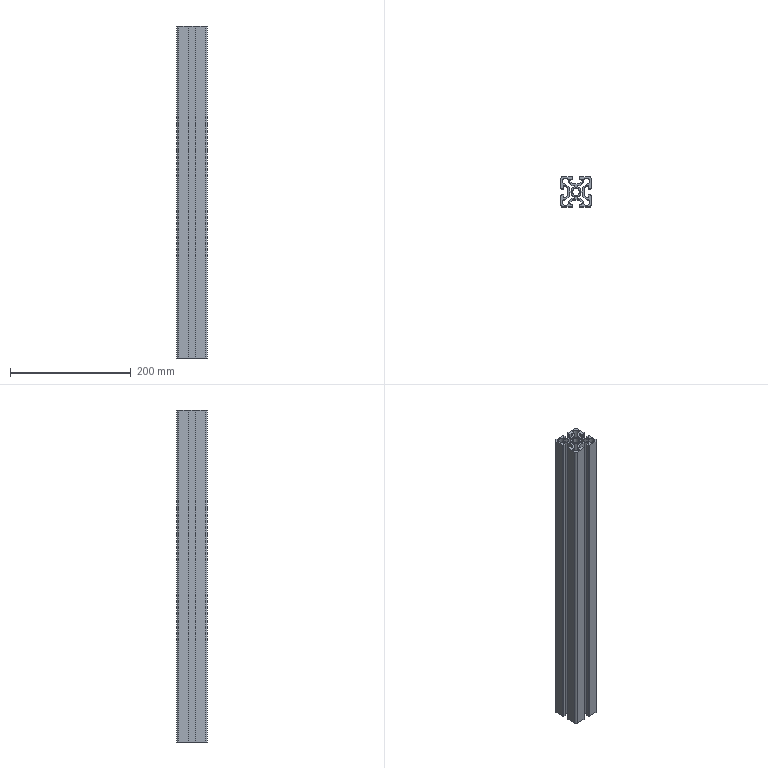Part | NX | features BREP 1 | 1 solid | 147 faces | box 50 x 50 x 550 mm | volume 544737 mm3 | plane 94 | cylinder 53 | commonest cylinder face diameters 2 x29 10 x12 6 x4 12 x4 17 x4